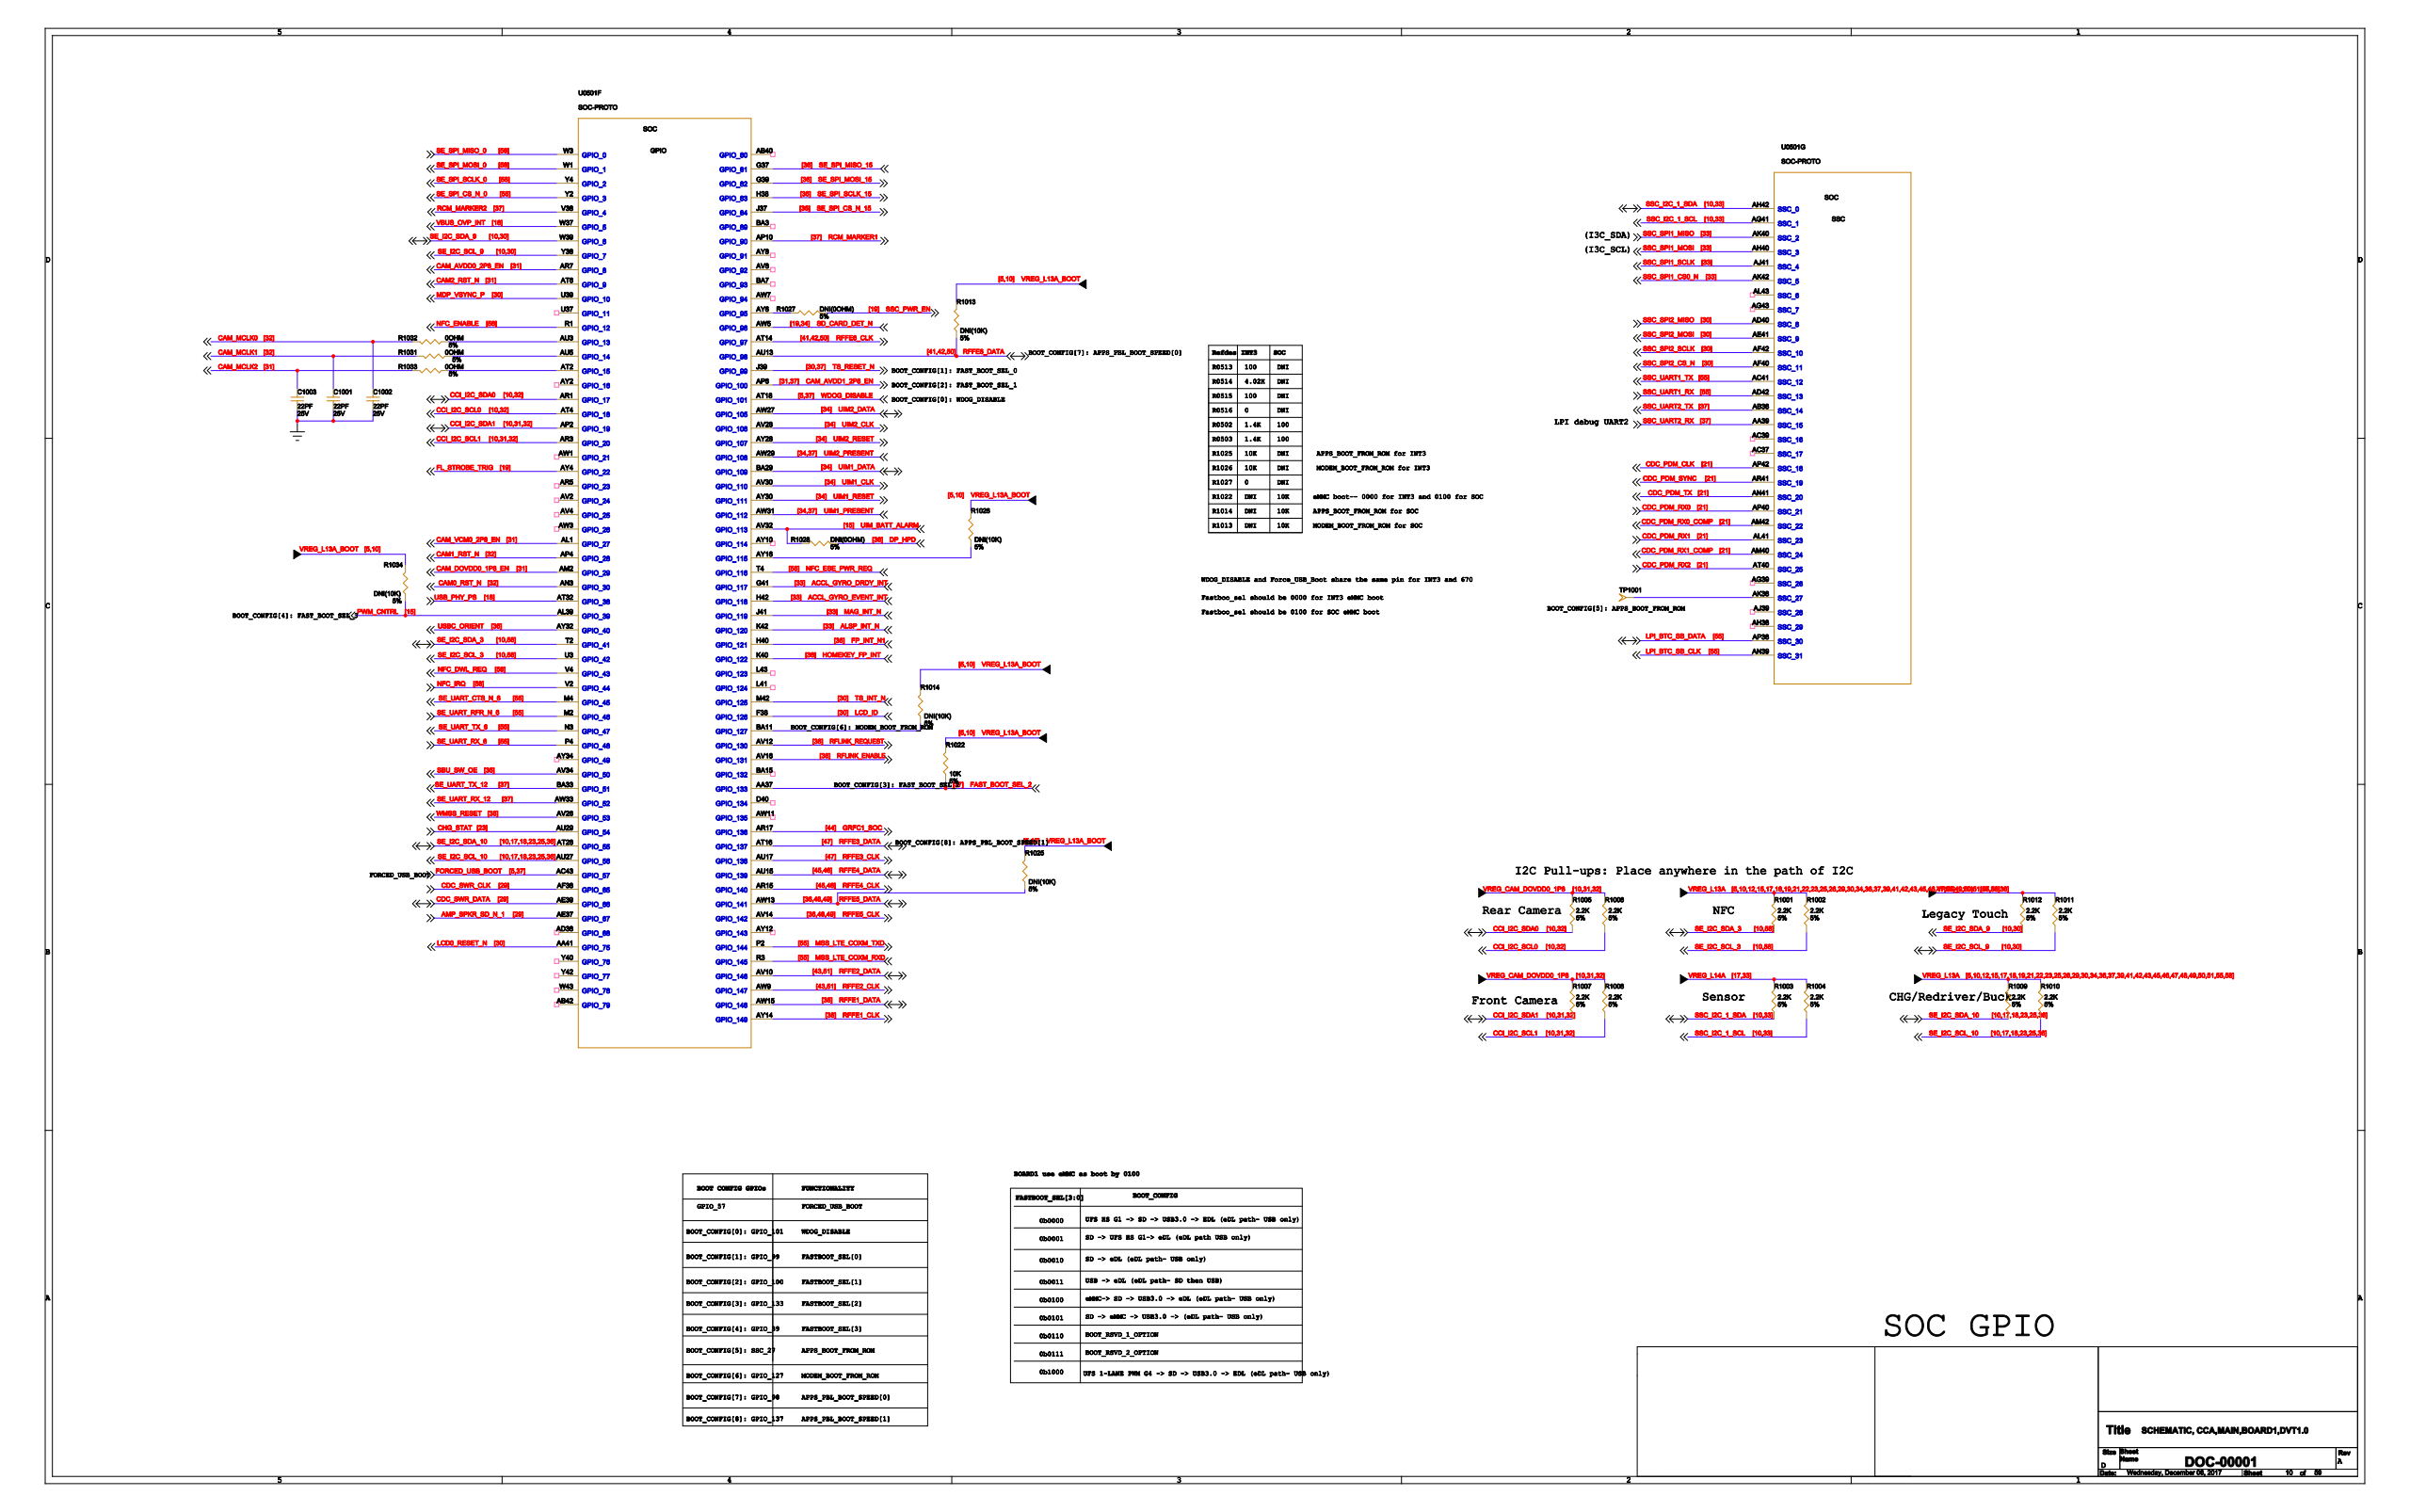Circuit board | KiCad | 1657 parts | 1365 nets | one sheet of the schematic
Parts on this sheet (reference | value | footprint):
C1001
C1002
C1003
R1001
R1002
R1003
R1004
R1005
R1006
R1007
R1008
R1009
R1010
R1011
R1012
R1013
R1025
R1027
R1028
R1031
R1032
R1033
R1034
TP1001
U0501
Nets of these parts (net: part-pin ...):
GND: C1001-2 C1002-2 C1003-2
N24160694: TP1001-1 U0501-AK38
VREG_L13A: R1001-1 R1002-1 R1009-1 R1010-1
VREG_L13A_BOOT: R1013-1 R1025-1 R1034-1
UIM1_CLK: U0501-AV30
SD_CARD_DET_N: U0501-AW5
RFFE2_CLK: U0501-AW9
RFFE6_DATA: R1013-2 U0501-AU13
VREG_L14A: R1003-1 R1004-1
TS_INT_N: U0501-M42
UIM2_CLK: U0501-AV28
RFFE6_CLK: U0501-AT14
SSC_SPI1_MOSI: U0501-AH40
VBUS_OVP_INT: U0501-W37
SE_I2C_SCL_10: R1010-2 U0501-AU27
SE_I2C_SDA_10: R1009-2 U0501-AT28
CAM_DOVDD0_1P8: R1005-1 R1006-1 R1007-1 R1008-1
CCI_I2C_SCL0: R1006-2 U0501-AT4
LCD0_RESET_N: U0501-AA41
SSC_SPI2_SCLK: U0501-AF42
VREG_L11A: R1011-1 R1012-1
RFFE5_DATA: R1025-2 U0501-AW13
UIM2_RESET: U0501-AY28
CDC_SWR_DATA: U0501-AE39
CAM_MCLK2: C1003-1 R1033-1
TS_RESET_N: U0501-J39
CCI_I2C_SDA1: R1007-2 U0501-AP2
RFFE2_DATA: U0501-AV10
WDOG_DISABLE: U0501-AT18
SE_I2C_SDA_9: R1012-2 U0501-W39
SE_I2C_SDA_3: R1001-2 U0501-T2
SSC_I2C_1_SDA: R1003-2 U0501-AH42
DP_HPD: R1028-1
UIM_BATT_ALARM: R1028-2 U0501-AV32
SBU_SW_OE: U0501-AV34
SSC_SPI1_MISO: U0501-AK40
SSC_UART1_RX: U0501-AD42
SSC_UART1_TX: U0501-AC41
LPI_BTC_SB_CLK: U0501-AN39
SE_UART_TX_6: U0501-N3
SE_UART_RX_6: U0501-P4
UIM1_RESET: U0501-AY30
CCI_I2C_SCL1: R1008-2 U0501-AR3
SE_I2C_SCL_3: R1002-2 U0501-U3
SE_I2C_SCL_9: R1011-2 U0501-Y38
CAM_MCLK1: C1001-1 R1031-1
SSC_SPI1_SCLK: U0501-AJ41
UIM1_PRESENT: U0501-AW31
UIM2_DATA: U0501-AW27
PWM_CNTRL: R1034-2 U0501-AL39
UIM1_DATA: U0501-BA29
SSC_SPI2_CS_N: U0501-AF40
CDC_SWR_CLK: U0501-AF38
SSC_SPI2_MISO: U0501-AD40
N24158270: R1031-2 U0501-AU5
CAM_MCLK0: C1002-1 R1032-1
CHG_STAT: U0501-AU29
SSC_SPI2_MOSI: U0501-AE41
SSC_UART2_RX: U0501-AA39
SSC_UART2_TX: U0501-AB38
SSC_I2C_1_SCL: R1004-2 U0501-AG41
SSC_SPI1_CS0_N: U0501-AK42
CDC_PDM_RX1: U0501-AL41
CAM0_RST_N: U0501-AN3
CDC_PDM_TX: U0501-AN41
CAM1_RST_N: U0501-AP4
RCM_MARKER1: U0501-AP10
CDC_PDM_RX0: U0501-AP40
CDC_PDM_CLK: U0501-AP42
CCI_I2C_SDA0: R1005-2 U0501-AR1
RFFE4_CLK: U0501-AR15
GRFC1_SOC: U0501-AR17
CDC_PDM_SYNC: U0501-AR41
N24158272: R1033-2 U0501-AT2
CAM2_RST_N: U0501-AT6
RFFE3_DATA: U0501-AT16
USB_PHY_PS: U0501-AT32
CDC_PDM_RX2: U0501-AT40
N24158268: R1032-2 U0501-AU3
RFFE4_DATA: U0501-AU15
RFFE3_CLK: U0501-AU17
RFLINK_REQUEST: U0501-AV12
RFFE5_CLK: U0501-AV14
RFLINK_ENABLE: U0501-AV16
WMSS_RESET: U0501-AV26
RFFE1_DATA: U0501-AW15
UIM2_PRESENT: U0501-AW29
SE_UART_RX_12: U0501-AW33
FL_STROBE_TRIG: U0501-AY4
N23068439: R1027-2 U0501-AY6
RFFE1_CLK: U0501-AY14
USBC_ORIENT: U0501-AY32
SE_UART_TX_12: U0501-BA33
LCD_ID: U0501-F38
SE_SPI_MISO_15: U0501-G37
SE_SPI_MOSI_15: U0501-G39
SE_SPI_SCLK_15: U0501-H38
FP_INT_N1: U0501-H40
SE_SPI_CS_N_15: U0501-J37
MAG_INT_N: U0501-J41
HOMEKEY_FP_INT: U0501-K40
ALSP_INT_N: U0501-K42
NFC_ENABLE: U0501-R1
MDP_VSYNC_P: U0501-U39
NFC_IRQ: U0501-V2
NFC_DWL_REQ: U0501-V4
RCM_MARKER2: U0501-V38
SE_SPI_MOSI_0: U0501-W1
SE_SPI_MISO_0: U0501-W3
SE_SPI_CS_N_0: U0501-Y2
SE_SPI_SCLK_0: U0501-Y4
SSC_PWR_EN: R1027-1